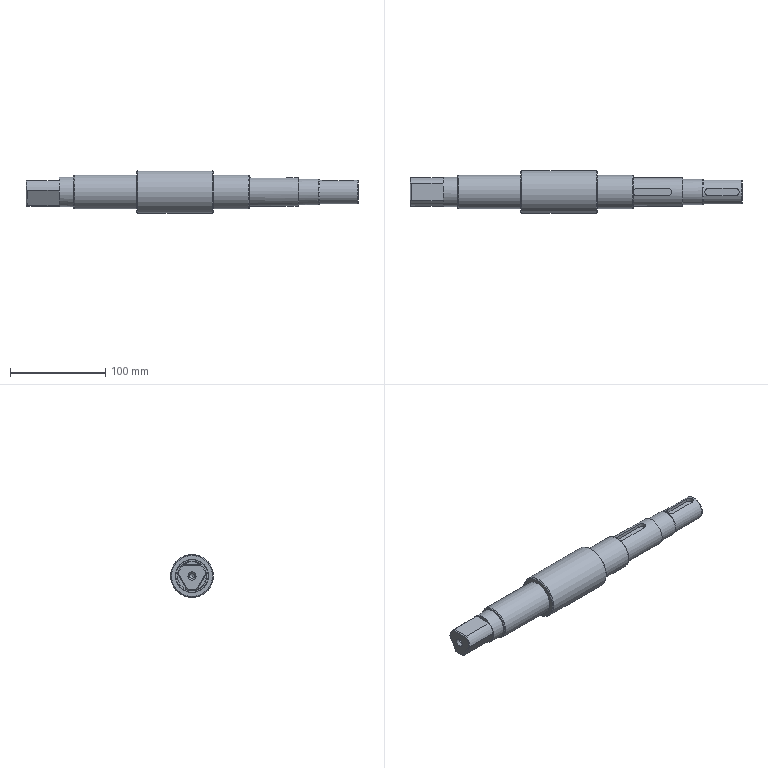NC program | NX | posted with a generic post | part box 348.4 x 45 x 45 mm
Lines 1 to 25 of 8230:
N10 G17 G21 G94 G90
(DRILLING , TOOL : ZXZ)
N12 T01 M6
N14 G54
N16 G17 G0 G90 X0. Y0. B0. C0. S5000 M3
N18 G43 Z30. H1
N20 G94 G81 G98 Z-1. F250. R3.
N22 G80
N24 G0 X0. Y0. Z30.
N26 M5
(DRILLING_COPY_COPY_1 , TOOL : 5.0ZT)
N28 T15 M6
N30 G54
N32 G17 G0 G90 X0. Y0. B0. C0. S2000 M3
N34 G43 Z30. H15
N36 G94 G83 G98 Z-24.502 F150. Q2. R3.
N38 G80
N40 G0 X0. Y0. Z30.
N42 M5